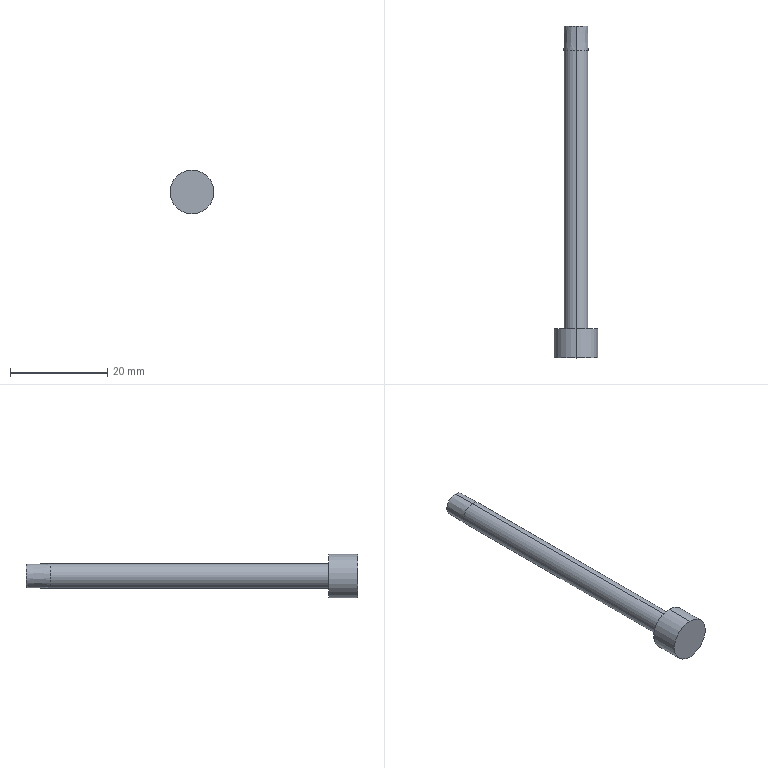Part | STEP file | 1 solid | 9 faces | box 9 x 68.14 x 9 mm | volume 1598 mm3 | cylinder 4 | plane 3 | cone 2 | commonest cylinder face diameters 5 x2 9 x2
STEP:
#1=CARTESIAN_POINT('',(0.,0.,0.));
#2=DIRECTION('',(0.,0.,1.));
#3=DIRECTION('',(1.,0.,0.));
#4=AXIS2_PLACEMENT_3D('',#1,#2,#3);
#5=CARTESIAN_POINT('',(-65.325,-40.,189.923));
#6=VERTEX_POINT('',#5);
#7=CARTESIAN_POINT('',(-65.325,-40.,180.923));
#8=VERTEX_POINT('',#7);
#9=CARTESIAN_POINT('',(-65.325,-40.,185.423));
#10=DIRECTION('',(0.,1.,0.));
#11=DIRECTION('',(0.,0.,-1.));
#12=AXIS2_PLACEMENT_3D('',#9,#10,#11);
#13=CIRCLE('',#12,4.5);
#14=CARTESIAN_POINT('',(-65.325,-50.,185.423));
#15=DIRECTION('',(0.,1.,0.));
#16=DIRECTION('',(0.,0.,1.));
#17=AXIS2_PLACEMENT_3D('',#14,#15,#16);
#18=CYLINDRICAL_SURFACE('',#17,4.5);
#19=CARTESIAN_POINT('',(-3.142,10.));
#20=DIRECTION('',(1.,0.));
#21=VECTOR('',#20,1.);
#22=LINE('',#19,#21);
#23=(GEOMETRIC_REPRESENTATION_CONTEXT(2)PARAMETRIC_REPRESENTATION_CONTEXT()REPRESENTATION_CONTEXT('',''));
#24=DEFINITIONAL_REPRESENTATION('',(#22),#23);
#25=PCURVE('',#18,#24);
#26=CARTESIAN_POINT('',(-72.862,-40.,23.556));
#27=DIRECTION('',(0.,-1.,0.));
#28=DIRECTION('',(0.,0.,-1.));
#29=AXIS2_PLACEMENT_3D('',#26,#27,#28);
#30=PLANE('',#29);
#31=CARTESIAN_POINT('',(-157.367,7.537));
#32=CARTESIAN_POINT('',(-157.367,-0.2567));
#33=CARTESIAN_POINT('',(-164.117,3.64));
#34=CARTESIAN_POINT('',(-170.867,7.537));
#35=CARTESIAN_POINT('',(-164.117,11.435));
#36=CARTESIAN_POINT('',(-157.367,15.332));
#37=CARTESIAN_POINT('',(-157.367,7.537));
#38=(BOUNDED_CURVE()B_SPLINE_CURVE(2,(#31,#32,#33,#34,#35,#36,#37),.UNSPECIFIED.,.T.,.F.)B_SPLINE_CURVE_WITH_KNOTS((1,2,2,2,2,1),(-2.094,0.,2.094,4.189,6.283,8.378),.UNSPECIFIED.)CURVE()GEOMETRIC_REPRESENTATION_ITEM()RATIONAL_B_SPLINE_CURVE((1.,0.5,1.,0.5,1.,0.5,1.))REPRESENTATION_ITEM(''));
#39=(GEOMETRIC_REPRESENTATION_CONTEXT(2)PARAMETRIC_REPRESENTATION_CONTEXT()REPRESENTATION_CONTEXT('',''));
#40=DEFINITIONAL_REPRESENTATION('',(#38),#39);
#41=PCURVE('',#30,#40);
#42=SURFACE_CURVE('',#13,(#25,#41),.PCURVE_S1.);
#43=EDGE_CURVE('',#6,#8,#42,.T.);
#44=ORIENTED_EDGE('',*,*,#43,.T.);
#45=CARTESIAN_POINT('',(-65.325,-34.,180.923));
#46=VERTEX_POINT('',#45);
#47=CARTESIAN_POINT('',(-65.325,-50.,180.923));
#48=DIRECTION('',(0.,1.,0.));
#49=VECTOR('',#48,1.);
#50=LINE('',#47,#49);
#51=CARTESIAN_POINT('',(3.142,0.));
#52=DIRECTION('',(0.,1.));
#53=VECTOR('',#52,1.);
#54=LINE('',#51,#53);
#55=(GEOMETRIC_REPRESENTATION_CONTEXT(2)PARAMETRIC_REPRESENTATION_CONTEXT()REPRESENTATION_CONTEXT('',''));
#56=DEFINITIONAL_REPRESENTATION('',(#54),#55);
#57=PCURVE('',#18,#56);
#58=CARTESIAN_POINT('',(-65.325,-50.,185.423));
#59=DIRECTION('',(0.,1.,0.));
#60=DIRECTION('',(0.,0.,1.));
#61=AXIS2_PLACEMENT_3D('',#58,#59,#60);
#62=CYLINDRICAL_SURFACE('',#61,4.5);
#63=CARTESIAN_POINT('',(3.142,0.));
#64=DIRECTION('',(0.,1.));
#65=VECTOR('',#64,1.);
#66=LINE('',#63,#65);
#67=(GEOMETRIC_REPRESENTATION_CONTEXT(2)PARAMETRIC_REPRESENTATION_CONTEXT()REPRESENTATION_CONTEXT('',''));
#68=DEFINITIONAL_REPRESENTATION('',(#66),#67);
#69=PCURVE('',#62,#68);
#70=SURFACE_CURVE('',#50,(#57,#69),.PCURVE_S1.);
#71=EDGE_CURVE('',#8,#46,#70,.T.);
#72=ORIENTED_EDGE('',*,*,#71,.T.);
#73=CARTESIAN_POINT('',(-65.325,-34.,189.923));
#74=VERTEX_POINT('',#73);
#75=CARTESIAN_POINT('',(-65.325,-34.,185.423));
#76=DIRECTION('',(0.,-1.,0.));
#77=DIRECTION('',(0.,0.,-1.));
#78=AXIS2_PLACEMENT_3D('',#75,#76,#77);
#79=CIRCLE('',#78,4.5);
#80=CARTESIAN_POINT('',(3.142,16.));
#81=DIRECTION('',(-1.,0.));
#82=VECTOR('',#81,1.);
#83=LINE('',#80,#82);
#84=(GEOMETRIC_REPRESENTATION_CONTEXT(2)PARAMETRIC_REPRESENTATION_CONTEXT()REPRESENTATION_CONTEXT('',''));
#85=DEFINITIONAL_REPRESENTATION('',(#83),#84);
#86=PCURVE('',#18,#85);
#87=CARTESIAN_POINT('',(-65.325,-34.,185.423));
#88=DIRECTION('',(0.,1.,0.));
#89=DIRECTION('',(0.,0.,1.));
#90=AXIS2_PLACEMENT_3D('',#87,#88,#89);
#91=PLANE('',#90);
#92=CARTESIAN_POINT('',(-4.5,0.));
#93=CARTESIAN_POINT('',(-4.5,7.794));
#94=CARTESIAN_POINT('',(2.25,3.897));
#95=CARTESIAN_POINT('',(9.,0.));
#96=CARTESIAN_POINT('',(2.25,-3.897));
#97=CARTESIAN_POINT('',(-4.5,-7.794));
#98=CARTESIAN_POINT('',(-4.5,0.));
#99=(BOUNDED_CURVE()B_SPLINE_CURVE(2,(#92,#93,#94,#95,#96,#97,#98),.UNSPECIFIED.,.T.,.F.)B_SPLINE_CURVE_WITH_KNOTS((1,2,2,2,2,1),(-2.094,0.,2.094,4.189,6.283,8.378),.UNSPECIFIED.)CURVE()GEOMETRIC_REPRESENTATION_ITEM()RATIONAL_B_SPLINE_CURVE((1.,0.5,1.,0.5,1.,0.5,1.))REPRESENTATION_ITEM(''));
#100=(GEOMETRIC_REPRESENTATION_CONTEXT(2)PARAMETRIC_REPRESENTATION_CONTEXT()REPRESENTATION_CONTEXT('',''));
#101=DEFINITIONAL_REPRESENTATION('',(#99),#100);
#102=PCURVE('',#91,#101);
#103=SURFACE_CURVE('',#79,(#86,#102),.PCURVE_S1.);
#104=EDGE_CURVE('',#46,#74,#103,.T.);
#105=ORIENTED_EDGE('',*,*,#104,.T.);
#106=CARTESIAN_POINT('',(-65.325,-50.,189.923));
#107=DIRECTION('',(0.,1.,0.));
#108=VECTOR('',#107,1.);
#109=LINE('',#106,#108);
#110=CARTESIAN_POINT('',(0.,0.));
#111=DIRECTION('',(0.,1.));
#112=VECTOR('',#111,1.);
#113=LINE('',#110,#112);
#114=(GEOMETRIC_REPRESENTATION_CONTEXT(2)PARAMETRIC_REPRESENTATION_CONTEXT()REPRESENTATION_CONTEXT('',''));
#115=DEFINITIONAL_REPRESENTATION('',(#113),#114);
#116=PCURVE('',#18,#115);
#117=CARTESIAN_POINT('',(6.283,0.));
#118=DIRECTION('',(0.,1.));
#119=VECTOR('',#118,1.);
#120=LINE('',#117,#119);
#121=(GEOMETRIC_REPRESENTATION_CONTEXT(2)PARAMETRIC_REPRESENTATION_CONTEXT()REPRESENTATION_CONTEXT('',''));
#122=DEFINITIONAL_REPRESENTATION('',(#120),#121);
#123=PCURVE('',#62,#122);
#124=SURFACE_CURVE('',#109,(#116,#123),.PCURVE_S1.);
#125=EDGE_CURVE('',#6,#74,#124,.T.);
#126=ORIENTED_EDGE('',*,*,#125,.F.);
#127=EDGE_LOOP('',(#44,#72,#105,#126));
#128=FACE_BOUND('',#127,.T.);
#129=ADVANCED_FACE('',(#128),#18,.T.);
#130=CARTESIAN_POINT('',(-65.325,28.14,187.835));
#131=VERTEX_POINT('',#130);
#132=CARTESIAN_POINT('',(-65.325,28.14,183.01));
#133=VERTEX_POINT('',#132);
#134=CARTESIAN_POINT('',(-65.325,28.14,185.423));
#135=DIRECTION('',(0.,1.,0.));
#136=DIRECTION('',(0.,0.,-1.));
#137=AXIS2_PLACEMENT_3D('',#134,#135,#136);
#138=CIRCLE('',#137,2.413);
#139=CARTESIAN_POINT('',(-65.325,22.412,185.423));
#140=DIRECTION('',(0.,-1.,0.));
#141=DIRECTION('',(0.,0.,-1.));
#142=AXIS2_PLACEMENT_3D('',#139,#140,#141);
#143=CONICAL_SURFACE('',#142,2.513,0.01745);
#144=CARTESIAN_POINT('',(6.283,-5.729));
#145=DIRECTION('',(-1.,0.));
#146=VECTOR('',#145,1.);
#147=LINE('',#144,#146);
#148=(GEOMETRIC_REPRESENTATION_CONTEXT(2)PARAMETRIC_REPRESENTATION_CONTEXT()REPRESENTATION_CONTEXT('',''));
#149=DEFINITIONAL_REPRESENTATION('',(#147),#148);
#150=PCURVE('',#143,#149);
#151=CARTESIAN_POINT('',(-65.325,28.14,185.423));
#152=DIRECTION('',(0.,1.,0.));
#153=DIRECTION('',(0.,0.,1.));
#154=AXIS2_PLACEMENT_3D('',#151,#152,#153);
#155=PLANE('',#154);
#156=CARTESIAN_POINT('',(0.,0.));
#157=DIRECTION('',(-1.,0.));
#158=AXIS2_PLACEMENT_2D('',#156,#157);
#159=CIRCLE('',#158,2.413);
#160=(GEOMETRIC_REPRESENTATION_CONTEXT(2)PARAMETRIC_REPRESENTATION_CONTEXT()REPRESENTATION_CONTEXT('',''));
#161=DEFINITIONAL_REPRESENTATION('',(#159),#160);
#162=PCURVE('',#155,#161);
#163=SURFACE_CURVE('',#138,(#150,#162),.PCURVE_S1.);
#164=EDGE_CURVE('',#131,#133,#163,.T.);
#165=ORIENTED_EDGE('',*,*,#164,.F.);
#166=CARTESIAN_POINT('',(-65.325,23.128,187.923));
#167=VERTEX_POINT('',#166);
#168=CARTESIAN_POINT('',(-65.325,22.412,187.935));
#169=DIRECTION('',(0.,-0.9998,0.01745));
#170=VECTOR('',#169,1.);
#171=LINE('',#168,#170);
#172=CARTESIAN_POINT('',(3.142,0.));
#173=DIRECTION('',(0.,1.));
#174=VECTOR('',#173,1.);
#175=LINE('',#172,#174);
#176=(GEOMETRIC_REPRESENTATION_CONTEXT(2)PARAMETRIC_REPRESENTATION_CONTEXT()REPRESENTATION_CONTEXT('',''));
#177=DEFINITIONAL_REPRESENTATION('',(#175),#176);
#178=PCURVE('',#143,#177);
#179=CARTESIAN_POINT('',(-65.325,22.412,185.423));
#180=DIRECTION('',(0.,-1.,0.));
#181=DIRECTION('',(0.,0.,-1.));
#182=AXIS2_PLACEMENT_3D('',#179,#180,#181);
#183=CONICAL_SURFACE('',#182,2.513,0.01745);
#184=CARTESIAN_POINT('',(3.142,0.));
#185=DIRECTION('',(0.,1.));
#186=VECTOR('',#185,1.);
#187=LINE('',#184,#186);
#188=(GEOMETRIC_REPRESENTATION_CONTEXT(2)PARAMETRIC_REPRESENTATION_CONTEXT()REPRESENTATION_CONTEXT('',''));
#189=DEFINITIONAL_REPRESENTATION('',(#187),#188);
#190=PCURVE('',#183,#189);
#191=SURFACE_CURVE('',#171,(#178,#190),.PCURVE_S1.);
#192=EDGE_CURVE('',#131,#167,#191,.T.);
#193=ORIENTED_EDGE('',*,*,#192,.T.);
#194=CARTESIAN_POINT('',(-65.325,23.128,182.923));
#195=VERTEX_POINT('',#194);
#196=CARTESIAN_POINT('',(-65.325,23.128,185.423));
#197=DIRECTION('',(0.,-1.,0.));
#198=DIRECTION('',(0.,0.,-1.));
#199=AXIS2_PLACEMENT_3D('',#196,#197,#198);
#200=CIRCLE('',#199,2.5);
#201=CARTESIAN_POINT('',(0.,-0.7161));
#202=DIRECTION('',(1.,0.));
#203=VECTOR('',#202,1.);
#204=LINE('',#201,#203);
#205=(GEOMETRIC_REPRESENTATION_CONTEXT(2)PARAMETRIC_REPRESENTATION_CONTEXT()REPRESENTATION_CONTEXT('',''));
#206=DEFINITIONAL_REPRESENTATION('',(#204),#205);
#207=PCURVE('',#143,#206);
#208=CARTESIAN_POINT('',(-65.325,28.14,185.423));
#209=DIRECTION('',(0.,-1.,0.));
#210=DIRECTION('',(0.,0.,-1.));
#211=AXIS2_PLACEMENT_3D('',#208,#209,#210);
#212=CYLINDRICAL_SURFACE('',#211,2.5);
#213=CARTESIAN_POINT('',(0.,5.012));
#214=DIRECTION('',(1.,0.));
#215=VECTOR('',#214,1.);
#216=LINE('',#213,#215);
#217=(GEOMETRIC_REPRESENTATION_CONTEXT(2)PARAMETRIC_REPRESENTATION_CONTEXT()REPRESENTATION_CONTEXT('',''));
#218=DEFINITIONAL_REPRESENTATION('',(#216),#217);
#219=PCURVE('',#212,#218);
#220=SURFACE_CURVE('',#200,(#207,#219),.PCURVE_S1.);
#221=EDGE_CURVE('',#195,#167,#220,.T.);
#222=ORIENTED_EDGE('',*,*,#221,.F.);
#223=CARTESIAN_POINT('',(-65.325,22.412,182.91));
#224=DIRECTION('',(0.,-0.9998,-0.01745));
#225=VECTOR('',#224,1.);
#226=LINE('',#223,#225);
#227=CARTESIAN_POINT('',(0.,0.));
#228=DIRECTION('',(0.,1.));
#229=VECTOR('',#228,1.);
#230=LINE('',#227,#229);
#231=(GEOMETRIC_REPRESENTATION_CONTEXT(2)PARAMETRIC_REPRESENTATION_CONTEXT()REPRESENTATION_CONTEXT('',''));
#232=DEFINITIONAL_REPRESENTATION('',(#230),#231);
#233=PCURVE('',#143,#232);
#234=CARTESIAN_POINT('',(6.283,0.));
#235=DIRECTION('',(0.,1.));
#236=VECTOR('',#235,1.);
#237=LINE('',#234,#236);
#238=(GEOMETRIC_REPRESENTATION_CONTEXT(2)PARAMETRIC_REPRESENTATION_CONTEXT()REPRESENTATION_CONTEXT('',''));
#239=DEFINITIONAL_REPRESENTATION('',(#237),#238);
#240=PCURVE('',#183,#239);
#241=SURFACE_CURVE('',#226,(#233,#240),.PCURVE_S1.);
#242=EDGE_CURVE('',#133,#195,#241,.T.);
#243=ORIENTED_EDGE('',*,*,#242,.F.);
#244=EDGE_LOOP('',(#165,#193,#222,#243));
#245=FACE_BOUND('',#244,.T.);
#246=ADVANCED_FACE('',(#245),#143,.T.);
#247=ORIENTED_EDGE('',*,*,#221,.T.);
#248=CARTESIAN_POINT('',(-65.325,-34.,187.923));
#249=VERTEX_POINT('',#248);
#250=CARTESIAN_POINT('',(-65.325,28.14,187.923));
#251=DIRECTION('',(0.,-1.,0.));
#252=VECTOR('',#251,1.);
#253=LINE('',#250,#252);
#254=CARTESIAN_POINT('',(3.142,0.));
#255=DIRECTION('',(0.,1.));
#256=VECTOR('',#255,1.);
#257=LINE('',#254,#256);
#258=(GEOMETRIC_REPRESENTATION_CONTEXT(2)PARAMETRIC_REPRESENTATION_CONTEXT()REPRESENTATION_CONTEXT('',''));
#259=DEFINITIONAL_REPRESENTATION('',(#257),#258);
#260=PCURVE('',#212,#259);
#261=CARTESIAN_POINT('',(-65.325,28.14,185.423));
#262=DIRECTION('',(0.,-1.,0.));
#263=DIRECTION('',(0.,0.,-1.));
#264=AXIS2_PLACEMENT_3D('',#261,#262,#263);
#265=CYLINDRICAL_SURFACE('',#264,2.5);
#266=CARTESIAN_POINT('',(3.142,0.));
#267=DIRECTION('',(0.,1.));
#268=VECTOR('',#267,1.);
#269=LINE('',#266,#268);
#270=(GEOMETRIC_REPRESENTATION_CONTEXT(2)PARAMETRIC_REPRESENTATION_CONTEXT()REPRESENTATION_CONTEXT('',''));
#271=DEFINITIONAL_REPRESENTATION('',(#269),#270);
#272=PCURVE('',#265,#271);
#273=SURFACE_CURVE('',#253,(#260,#272),.PCURVE_S1.);
#274=EDGE_CURVE('',#167,#249,#273,.T.);
#275=ORIENTED_EDGE('',*,*,#274,.T.);
#276=CARTESIAN_POINT('',(-65.325,-34.,182.923));
#277=VERTEX_POINT('',#276);
#278=CARTESIAN_POINT('',(-65.325,-34.,185.423));
#279=DIRECTION('',(0.,-1.,0.));
#280=DIRECTION('',(0.,0.,1.));
#281=AXIS2_PLACEMENT_3D('',#278,#279,#280);
#282=CIRCLE('',#281,2.5);
#283=CARTESIAN_POINT('',(-3.142,62.14));
#284=DIRECTION('',(1.,0.));
#285=VECTOR('',#284,1.);
#286=LINE('',#283,#285);
#287=(GEOMETRIC_REPRESENTATION_CONTEXT(2)PARAMETRIC_REPRESENTATION_CONTEXT()REPRESENTATION_CONTEXT('',''));
#288=DEFINITIONAL_REPRESENTATION('',(#286),#287);
#289=PCURVE('',#212,#288);
#290=CARTESIAN_POINT('',(2.5,0.));
#291=CARTESIAN_POINT('',(2.5,-4.33));
#292=CARTESIAN_POINT('',(-1.25,-2.165));
#293=CARTESIAN_POINT('',(-5.,0.));
#294=CARTESIAN_POINT('',(-1.25,2.165));
#295=CARTESIAN_POINT('',(2.5,4.33));
#296=CARTESIAN_POINT('',(2.5,0.));
#297=(BOUNDED_CURVE()B_SPLINE_CURVE(2,(#290,#291,#292,#293,#294,#295,#296),.UNSPECIFIED.,.T.,.F.)B_SPLINE_CURVE_WITH_KNOTS((1,2,2,2,2,1),(-2.094,0.,2.094,4.189,6.283,8.378),.UNSPECIFIED.)CURVE()GEOMETRIC_REPRESENTATION_ITEM()RATIONAL_B_SPLINE_CURVE((1.,0.5,1.,0.5,1.,0.5,1.))REPRESENTATION_ITEM(''));
#298=(GEOMETRIC_REPRESENTATION_CONTEXT(2)PARAMETRIC_REPRESENTATION_CONTEXT()REPRESENTATION_CONTEXT('',''));
#299=DEFINITIONAL_REPRESENTATION('',(#297),#298);
#300=PCURVE('',#91,#299);
#301=SURFACE_CURVE('',#282,(#289,#300),.PCURVE_S1.);
#302=EDGE_CURVE('',#277,#249,#301,.T.);
#303=ORIENTED_EDGE('',*,*,#302,.F.);
#304=CARTESIAN_POINT('',(-65.325,28.14,182.923));
#305=DIRECTION('',(0.,-1.,0.));
#306=VECTOR('',#305,1.);
#307=LINE('',#304,#306);
#308=CARTESIAN_POINT('',(0.,0.));
#309=DIRECTION('',(0.,1.));
#310=VECTOR('',#309,1.);
#311=LINE('',#308,#310);
#312=(GEOMETRIC_REPRESENTATION_CONTEXT(2)PARAMETRIC_REPRESENTATION_CONTEXT()REPRESENTATION_CONTEXT('',''));
#313=DEFINITIONAL_REPRESENTATION('',(#311),#312);
#314=PCURVE('',#212,#313);
#315=CARTESIAN_POINT('',(6.283,0.));
#316=DIRECTION('',(0.,1.));
#317=VECTOR('',#316,1.);
#318=LINE('',#315,#317);
#319=(GEOMETRIC_REPRESENTATION_CONTEXT(2)PARAMETRIC_REPRESENTATION_CONTEXT()REPRESENTATION_CONTEXT('',''));
#320=DEFINITIONAL_REPRESENTATION('',(#318),#319);
#321=PCURVE('',#265,#320);
#322=SURFACE_CURVE('',#307,(#314,#321),.PCURVE_S1.);
#323=EDGE_CURVE('',#195,#277,#322,.T.);
#324=ORIENTED_EDGE('',*,*,#323,.F.);
#325=EDGE_LOOP('',(#247,#275,#303,#324));
#326=FACE_BOUND('',#325,.T.);
#327=ADVANCED_FACE('',(#326),#212,.T.);
#328=ORIENTED_EDGE('',*,*,#274,.F.);
#329=CARTESIAN_POINT('',(-65.325,23.128,185.423));
#330=DIRECTION('',(0.,-1.,0.));
#331=DIRECTION('',(0.,0.,-1.));
#332=AXIS2_PLACEMENT_3D('',#329,#330,#331);
#333=CIRCLE('',#332,2.5);
#334=CARTESIAN_POINT('',(0.,5.012));
#335=DIRECTION('',(1.,0.));
#336=VECTOR('',#335,1.);
#337=LINE('',#334,#336);
#338=(GEOMETRIC_REPRESENTATION_CONTEXT(2)PARAMETRIC_REPRESENTATION_CONTEXT()REPRESENTATION_CONTEXT('',''));
#339=DEFINITIONAL_REPRESENTATION('',(#337),#338);
#340=PCURVE('',#265,#339);
#341=CARTESIAN_POINT('',(0.,-0.7161));
#342=DIRECTION('',(1.,0.));
#343=VECTOR('',#342,1.);
#344=LINE('',#341,#343);
#345=(GEOMETRIC_REPRESENTATION_CONTEXT(2)PARAMETRIC_REPRESENTATION_CONTEXT()REPRESENTATION_CONTEXT('',''));
#346=DEFINITIONAL_REPRESENTATION('',(#344),#345);
#347=PCURVE('',#183,#346);
#348=SURFACE_CURVE('',#333,(#340,#347),.PCURVE_S1.);
#349=EDGE_CURVE('',#167,#195,#348,.T.);
#350=ORIENTED_EDGE('',*,*,#349,.T.);
#351=ORIENTED_EDGE('',*,*,#323,.T.);
#352=CARTESIAN_POINT('',(-65.325,-34.,185.423));
#353=DIRECTION('',(0.,-1.,0.));
#354=DIRECTION('',(0.,0.,1.));
#355=AXIS2_PLACEMENT_3D('',#352,#353,#354);
#356=CIRCLE('',#355,2.5);
#357=CARTESIAN_POINT('',(3.142,62.14));
#358=DIRECTION('',(1.,0.));
#359=VECTOR('',#358,1.);
#360=LINE('',#357,#359);
#361=(GEOMETRIC_REPRESENTATION_CONTEXT(2)PARAMETRIC_REPRESENTATION_CONTEXT()REPRESENTATION_CONTEXT('',''));
#362=DEFINITIONAL_REPRESENTATION('',(#360),#361);
#363=PCURVE('',#265,#362);
#364=CARTESIAN_POINT('',(2.5,0.));
#365=CARTESIAN_POINT('',(2.5,-4.33));
#366=CARTESIAN_POINT('',(-1.25,-2.165));
#367=CARTESIAN_POINT('',(-5.,0.));
#368=CARTESIAN_POINT('',(-1.25,2.165));
#369=CARTESIAN_POINT('',(2.5,4.33));
#370=CARTESIAN_POINT('',(2.5,0.));
#371=(BOUNDED_CURVE()B_SPLINE_CURVE(2,(#364,#365,#366,#367,#368,#369,#370),.UNSPECIFIED.,.T.,.F.)B_SPLINE_CURVE_WITH_KNOTS((1,2,2,2,2,1),(-2.094,0.,2.094,4.189,6.283,8.378),.UNSPECIFIED.)CURVE()GEOMETRIC_REPRESENTATION_ITEM()RATIONAL_B_SPLINE_CURVE((1.,0.5,1.,0.5,1.,0.5,1.))REPRESENTATION_ITEM(''));
#372=(GEOMETRIC_REPRESENTATION_CONTEXT(2)PARAMETRIC_REPRESENTATION_CONTEXT()REPRESENTATION_CONTEXT('',''));
#373=DEFINITIONAL_REPRESENTATION('',(#371),#372);
#374=PCURVE('',#91,#373);
#375=SURFACE_CURVE('',#356,(#363,#374),.PCURVE_S1.);
#376=EDGE_CURVE('',#249,#277,#375,.T.);
#377=ORIENTED_EDGE('',*,*,#376,.F.);
#378=EDGE_LOOP('',(#328,#350,#351,#377));
#379=FACE_BOUND('',#378,.T.);
#380=ADVANCED_FACE('',(#379),#265,.T.);
#381=ORIENTED_EDGE('',*,*,#192,.F.);
#382=CARTESIAN_POINT('',(-65.325,28.14,185.423));
#383=DIRECTION('',(0.,1.,0.));
#384=DIRECTION('',(0.,0.,-1.));
#385=AXIS2_PLACEMENT_3D('',#382,#383,#384);
#386=CIRCLE('',#385,2.413);
#387=CARTESIAN_POINT('',(6.283,-5.729));
#388=DIRECTION('',(-1.,0.));
#389=VECTOR('',#388,1.);
#390=LINE('',#387,#389);
#391=(GEOMETRIC_REPRESENTATION_CONTEXT(2)PARAMETRIC_REPRESENTATION_CONTEXT()REPRESENTATION_CONTEXT('',''));
#392=DEFINITIONAL_REPRESENTATION('',(#390),#391);
#393=PCURVE('',#183,#392);
#394=CARTESIAN_POINT('',(0.,0.));
#395=DIRECTION('',(-1.,0.));
#396=AXIS2_PLACEMENT_2D('',#394,#395);
#397=CIRCLE('',#396,2.413);
#398=(GEOMETRIC_REPRESENTATION_CONTEXT(2)PARAMETRIC_REPRESENTATION_CONTEXT()REPRESENTATION_CONTEXT('',''));
#399=DEFINITIONAL_REPRESENTATION('',(#397),#398);
#400=PCURVE('',#155,#399);
#401=SURFACE_CURVE('',#386,(#393,#400),.PCURVE_S1.);
#402=EDGE_CURVE('',#133,#131,#401,.T.);
#403=ORIENTED_EDGE('',*,*,#402,.F.);
#404=ORIENTED_EDGE('',*,*,#242,.T.);
#405=ORIENTED_EDGE('',*,*,#349,.F.);
#406=EDGE_LOOP('',(#381,#403,#404,#405));
#407=FACE_BOUND('',#406,.T.);
#408=ADVANCED_FACE('',(#407),#183,.T.);
#409=ORIENTED_EDGE('',*,*,#402,.T.);
#410=ORIENTED_EDGE('',*,*,#164,.T.);
#411=EDGE_LOOP('',(#409,#410));
#412=FACE_BOUND('',#411,.T.);
#413=ADVANCED_FACE('',(#412),#155,.T.);
#414=ORIENTED_EDGE('',*,*,#302,.T.);
#415=ORIENTED_EDGE('',*,*,#376,.T.);
#416=EDGE_LOOP('',(#414,#415));
#417=FACE_BOUND('',#416,.T.);
#418=CARTESIAN_POINT('',(-65.325,-34.,185.423));
#419=DIRECTION('',(0.,-1.,0.));
#420=DIRECTION('',(0.,0.,-1.));
#421=AXIS2_PLACEMENT_3D('',#418,#419,#420);
#422=CIRCLE('',#421,4.5);
#423=CARTESIAN_POINT('',(-4.5,0.));
#424=CARTESIAN_POINT('',(-4.5,7.794));
#425=CARTESIAN_POINT('',(2.25,3.897));
#426=CARTESIAN_POINT('',(9.,0.));
#427=CARTESIAN_POINT('',(2.25,-3.897));
#428=CARTESIAN_POINT('',(-4.5,-7.794));
#429=CARTESIAN_POINT('',(-4.5,0.));
#430=(BOUNDED_CURVE()B_SPLINE_CURVE(2,(#423,#424,#425,#426,#427,#428,#429),.UNSPECIFIED.,.T.,.F.)B_SPLINE_CURVE_WITH_KNOTS((1,2,2,2,2,1),(-2.094,0.,2.094,4.189,6.283,8.378),.UNSPECIFIED.)CURVE()GEOMETRIC_REPRESENTATION_ITEM()RATIONAL_B_SPLINE_CURVE((1.,0.5,1.,0.5,1.,0.5,1.))REPRESENTATION_ITEM(''));
#431=(GEOMETRIC_REPRESENTATION_CONTEXT(2)PARAMETRIC_REPRESENTATION_CONTEXT()REPRESENTATION_CONTEXT('',''));
#432=DEFINITIONAL_REPRESENTATION('',(#430),#431);
#433=PCURVE('',#91,#432);
#434=CARTESIAN_POINT('',(9.425,16.));
#435=DIRECTION('',(-1.,0.));
#436=VECTOR('',#435,1.);
#437=LINE('',#434,#436);
#438=(GEOMETRIC_REPRESENTATION_CONTEXT(2)PARAMETRIC_REPRESENTATION_CONTEXT()REPRESENTATION_CONTEXT('',''));
#439=DEFINITIONAL_REPRESENTATION('',(#437),#438);
#440=PCURVE('',#62,#439);
#441=SURFACE_CURVE('',#422,(#433,#440),.PCURVE_S1.);
#442=EDGE_CURVE('',#74,#46,#441,.T.);
#443=ORIENTED_EDGE('',*,*,#442,.F.);
#444=ORIENTED_EDGE('',*,*,#104,.F.);
#445=EDGE_LOOP('',(#443,#444));
#446=FACE_BOUND('',#445,.T.);
#447=ADVANCED_FACE('',(#417,#446),#91,.T.);
#448=ORIENTED_EDGE('',*,*,#71,.F.);
#449=CARTESIAN_POINT('',(-65.325,-40.,185.423));
#450=DIRECTION('',(0.,1.,0.));
#451=DIRECTION('',(0.,0.,-1.));
#452=AXIS2_PLACEMENT_3D('',#449,#450,#451);
#453=CIRCLE('',#452,4.5);
#454=CARTESIAN_POINT('',(3.142,10.));
#455=DIRECTION('',(1.,0.));
#456=VECTOR('',#455,1.);
#457=LINE('',#454,#456);
#458=(GEOMETRIC_REPRESENTATION_CONTEXT(2)PARAMETRIC_REPRESENTATION_CONTEXT()REPRESENTATION_CONTEXT('',''));
#459=DEFINITIONAL_REPRESENTATION('',(#457),#458);
#460=PCURVE('',#62,#459);
#461=CARTESIAN_POINT('',(-157.367,7.537));
#462=CARTESIAN_POINT('',(-157.367,-0.2567));
#463=CARTESIAN_POINT('',(-164.117,3.64));
#464=CARTESIAN_POINT('',(-170.867,7.537));
#465=CARTESIAN_POINT('',(-164.117,11.435));
#466=CARTESIAN_POINT('',(-157.367,15.332));
#467=CARTESIAN_POINT('',(-157.367,7.537));
#468=(BOUNDED_CURVE()B_SPLINE_CURVE(2,(#461,#462,#463,#464,#465,#466,#467),.UNSPECIFIED.,.T.,.F.)B_SPLINE_CURVE_WITH_KNOTS((1,2,2,2,2,1),(-2.094,0.,2.094,4.189,6.283,8.378),.UNSPECIFIED.)CURVE()GEOMETRIC_REPRESENTATION_ITEM()RATIONAL_B_SPLINE_CURVE((1.,0.5,1.,0.5,1.,0.5,1.))REPRESENTATION_ITEM(''));
#469=(GEOMETRIC_REPRESENTATION_CONTEXT(2)PARAMETRIC_REPRESENTATION_CONTEXT()REPRESENTATION_CONTEXT('',''));
#470=DEFINITIONAL_REPRESENTATION('',(#468),#469);
#471=PCURVE('',#30,#470);
#472=SURFACE_CURVE('',#453,(#460,#471),.PCURVE_S1.);
#473=EDGE_CURVE('',#8,#6,#472,.T.);
#474=ORIENTED_EDGE('',*,*,#473,.T.);
#475=ORIENTED_EDGE('',*,*,#125,.T.);
#476=ORIENTED_EDGE('',*,*,#442,.T.);
#477=EDGE_LOOP('',(#448,#474,#475,#476));
#478=FACE_BOUND('',#477,.T.);
#479=ADVANCED_FACE('',(#478),#62,.T.);
#480=ORIENTED_EDGE('',*,*,#43,.F.);
#481=ORIENTED_EDGE('',*,*,#473,.F.);
#482=EDGE_LOOP('',(#480,#481));
#483=FACE_BOUND('',#482,.T.);
#484=ADVANCED_FACE('',(#483),#30,.T.);
#485=CLOSED_SHELL('',(#129,#246,#327,#380,#408,#413,#447,#479,#484));
#486=MANIFOLD_SOLID_BREP('',#485);
#487=(LENGTH_UNIT()NAMED_UNIT(*)SI_UNIT(.MILLI.,.METRE.));
#488=UNCERTAINTY_MEASURE_WITH_UNIT(LENGTH_MEASURE(0.0000001),#487,'','');
#489=(NAMED_UNIT(*)PLANE_ANGLE_UNIT()SI_UNIT($,.RADIAN.));
#490=(NAMED_UNIT(*)SI_UNIT($,.STERADIAN.)SOLID_ANGLE_UNIT());
#491=(GEOMETRIC_REPRESENTATION_CONTEXT(3)GLOBAL_UNCERTAINTY_ASSIGNED_CONTEXT((#488))GLOBAL_UNIT_ASSIGNED_CONTEXT((#487,#489,#490))REPRESENTATION_CONTEXT('',''));
#492=ADVANCED_BREP_SHAPE_REPRESENTATION('',(#4,#486),#491);